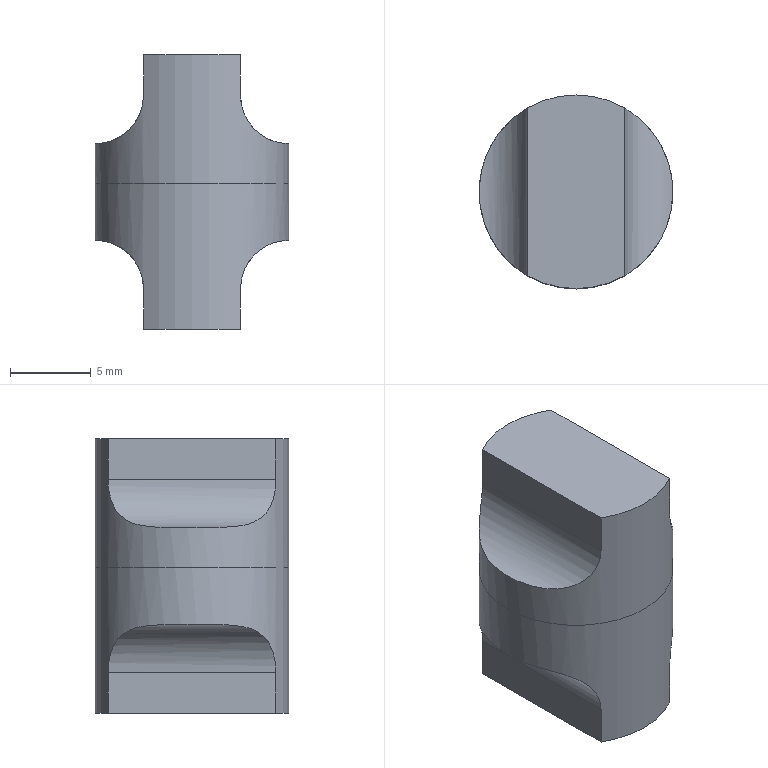NC program | NX | posted with a generic post | part box 12 x 12 x 17 mm
Lines 1210 to 2569 of 2569:
(PLANAR_MILL_COPY_1_COPY_COPY , TOOL : D8开粗)
N2328 T01 M6
N2330 G54
N2332 G17 G0 G90 X0. Y-12.196 S2000 M3
N2334 G43 Z20. H1
N2336 Z2.05
N2338 G94 G1 Z0.05 F800.
N2340 Y-5.196
N2342 Y5.196
N2344 Y12.196
N2346 Z2.05
N2348 G0 Z20.
(ADAPTIVE_MILLING_1_COPY , TOOL : D8开粗)
N2350 X-16.493 Y0.096 S2500
N2352 Z-6.994
N2354 G1 X-16.343 Z-7.931 F1000.
N2356 X-16.193 Z-8.301
N2358 X-16.043 Z-8.574
N2360 X-15.893 Z-8.794
N2362 X-15.743 Z-8.978
N2364 X-15.593 Z-9.136
N2366 X-15.443 Z-9.274
N2368 X-15.293 Z-9.394
N2370 X-15.143 Z-9.499
N2372 X-14.993 Z-9.592
N2374 X-14.843 Z-9.673
N2376 X-14.693 Z-9.743
N2378 X-14.543 Z-9.804
N2380 X-14.393 Z-9.856
N2382 X-14.243 Z-9.899
N2384 X-14.093 Z-9.933
N2386 X-13.943 Z-9.96
N2388 X-13.793 Z-9.979
N2390 X-13.643 Y0.095 Z-9.99
N2392 X-13.493 Z-9.994
N2394 X-12.229
N2396 G3 X-11.465 Y0.639 R0.809
N2398 G2 X-10.606 Y3.647 R33.117
N2400 X4.464 Y10.246 R11.261
N2402 X-11.107 Y-1.066 R-11.169
N2404 X-6.24 Y8.898 R11.713
N2406 X-10.604 Y-2.307 R-10.863
N2408 X-3.391 Y9.995 R11.018
N2410 X-10.105 Y-2.977 R-10.55
N2412 X-1.423 Y10.137 R10.58
N2414 X-9.548 Y-3.628 R-10.231
N2416 X-10.028 Y1.009 R9.78
N2418 X-9.875 Y2.002 R4.333
N2420 G1 X-9.695 Y2.83
N2422 G2 X-8.521 Y5.423 R11.812
N2424 X-6.668 Y7.586 R11.812
N2426 X-4.354 Y9.113 R11.863
N2428 X-0.441 Y10.09 R10.913
N2430 X3.543 Y9.458 R10.913
N2432 G1 X4.9 Y8.832
N2434 X6.149 Y8.012
N2436 X7.264 Y7.017
N2438 X8.22 Y5.868
N2440 X8.996 Y4.591
N2442 X9.575 Y3.213
N2444 X9.944 Y1.765
N2446 X10.096 Y0.279
N2448 X10.027 Y-1.214
N2450 X9.738 Y-2.68
N2452 X9.236 Y-4.088
N2454 X8.531 Y-5.406
N2456 X7.639 Y-6.607
N2458 X6.579 Y-7.663
N2460 G2 X5.058 Y-8.743 R18.614
N2462 G1 X3.65 Y-9.417
N2464 X2.174 Y-9.863
N2466 X0.646 Y-10.079
N2468 X-0.896 Y-10.06
N2470 X-2.418 Y-9.806
N2472 X-3.883 Y-9.323
N2474 X-5.258 Y-8.623
N2476 X-6.51 Y-7.722
N2478 X-7.61 Y-6.64
N2480 X-8.533 Y-5.404
N2482 G2 X-9.702 Y-2.808 R11.812
N2484 X-10.1 Y0.01 R11.818
N2486 G1 X-9.997 Y1.435
N2488 X-9.871 Y2.021
N2490 G3 X-10.332 Y2.931 R0.808
N2492 G1 X-11.574 Y3.482
N2494 X-11.711 Y3.543 Z-9.99
N2496 X-11.848 Y3.604 Z-9.979
N2498 X-11.985 Y3.665 Z-9.96
N2500 X-12.122 Y3.726 Z-9.933
N2502 X-12.259 Y3.787 Z-9.899
N2504 X-12.396 Y3.848 Z-9.856
N2506 X-12.534 Y3.909 Z-9.804
N2508 X-12.671 Y3.97 Z-9.743
N2510 X-12.808 Y4.031 Z-9.673
N2512 X-12.945 Y4.092 Z-9.592
N2514 X-13.082 Y4.152 Z-9.499
N2516 X-13.219 Y4.213 Z-9.394
N2518 X-13.356 Y4.274 Z-9.274
N2520 X-13.493 Y4.335 Z-9.136
N2522 X-13.63 Y4.396 Z-8.978
N2524 X-13.767 Y4.457 Z-8.794
N2526 X-13.904 Y4.518 Z-8.574
N2528 X-14.041 Y4.579 Z-8.301
N2530 X-14.178 Y4.64 Z-7.931
N2532 X-14.316 Y4.701 Z-6.994
N2534 G0 Z20.
N2536 X-10.972 Y-10.352
N2538 Z-1.997
N2540 G1 X-10.86 Y-10.252 Z-2.934
N2542 X-10.749 Y-10.151 Z-3.305
N2544 X-10.638 Y-10.051 Z-3.577
N2546 X-10.526 Y-9.95 Z-3.797
N2548 X-10.415 Y-9.85 Z-3.981
N2550 X-10.304 Y-9.749 Z-4.139
N2552 X-10.192 Y-9.649 Z-4.277
N2554 X-10.081 Y-9.548 Z-4.397
N2556 X-9.969 Y-9.448 Z-4.502
N2558 X-9.858 Y-9.347 Z-4.595
N2560 X-9.747 Y-9.247 Z-4.676
N2562 X-9.635 Y-9.146 Z-4.746
N2564 X-9.524 Y-9.046 Z-4.807
N2566 X-9.412 Y-8.945 Z-4.859
N2568 X-9.301 Y-8.845 Z-4.902
N2570 X-9.19 Y-8.745 Z-4.936
N2572 X-9.078 Y-8.644 Z-4.963
N2574 X-8.967 Y-8.544 Z-4.982
N2576 X-8.856 Y-8.443 Z-4.993
N2578 X-8.744 Y-8.343 Z-4.997
N2580 X-7.834 Y-7.521
N2582 G3 X-7.742 Y-6.419 R0.808
N2584 G2 X-9.589 Y-1.959 R13.939
N2586 X-8.36 Y5.047 R9.929
N2588 X-7.73 Y6.434 R4.2
N2590 G3 X-8.564 Y7.705 R0.8
N2592 X-8.986 Y7.449 Z-4.966 R1.078
N2594 G1 X-9.831 Y6.752 Z-4.897
N2596 X-10.469 Y6.225 F10000.
N2598 G3 X-10.759 Y5.623 R0.803
N2600 G1 X-10.954 Y-5.3
N2602 G3 X-10.641 Y-5.949 R0.802
N2604 G1 X-10.006 Y-6.437
N2606 X-9.072 Y-7.148 Z-4.971 F1000.
N2608 G3 X-8.68 Y-7.28 Z-4.997 R0.81
N2610 X-7.925 Y-6.112 R0.8
N2612 G2 X-8.398 Y-5.006 R5.111
N2614 X-9.449 Y-0.645 R13.912
N2616 X-8.524 Y4.104 R10.597
N2618 G1 X-8.442 Y4.768
N2620 X-8.35 Y5.08
N2622 G3 X-9.525 Y5.996 R0.8
N2624 X-9.874 Y5.607 Z-4.964 R1.031
N2626 G1 X-10.443 Y4.708 Z-4.897
N2628 X-10.724 Y4.27 F10000.
N2630 X-10.993 Y3.826
N2632 X-11.044 Y3.672
N2634 X-11.066 Y3.512
N2636 X-11.259 Y-4.672
N2638 G3 X-10.917 Y-5.348 R0.801
N2640 G1 X-10.213 Y-5.839
N2642 X-9.397 Y-6.401 Z-4.959 F1000.
N2644 G3 X-8.817 Y-6.491 Z-4.997 R0.801
N2646 X-8.23 Y-5.484 R0.8
N2648 G2 X-9.121 Y-1.322 R24.508
N2650 X-8.6 Y3.105 R11.126
N2652 G3 X-8.525 Y3.922 R2.117
N2654 G1 X-8.493 Y4.245
N2656 G3 X-9.346 Y5.121 R0.8
N2658 X-9.961 Y4.766 Z-4.951 R0.841
N2660 G1 X-10.501 Y4.098 Z-4.897
N2662 X-11.419 Y2.964 F10000.
N2664 G3 X-11.597 Y2.453 R0.807
N2666 G1 X-11.547 Y-2.973
N2668 G3 X-11.371 Y-3.467 R0.808
N2670 G1 X-10.47 Y-4.588
N2672 X-9.82 Y-5.389 Z-4.962 F1000.
N2674 G3 X-9.331 Y-5.638 Z-4.997 R0.802
N2676 X-8.443 Y-4.765 R0.8
N2678 X-8.829 Y-1.849 R153.035
N2680 G2 X-8.526 Y2.412 R13.535
N2682 G1 X-8.525 Y3.462
N2684 G3 X-9.318 Y4.262 R0.8
N2686 X-9.985 Y3.921 Z-4.948 R0.83
N2688 G1 X-10.51 Y3.297 Z-4.897
N2690 X-11.441 Y2.191 F10000.
N2692 G3 X-11.629 Y1.67 R0.807
N2694 G1 X-11.6 Y-2.426
N2696 G3 X-11.424 Y-2.922 R0.808
N2698 G1 X-10.519 Y-4.046
N2700 X-9.873 Y-4.843 Z-4.961 F1000.
N2702 G3 X-9.377 Y-5.091 Z-4.997 R0.802
N2704 X-8.496 Y-4.218 R0.8
N2706 G2 X-8.644 Y-0.765 R76.33
N2708 X-8.525 Y0.856 R32.63
N2710 G1 Y2.456
N2712 G3 X-9.901 Y3.011 R0.8
N2714 X-10.13 Y2.585 Z-4.966 R1.096
N2716 G1 X-10.512 Y1.549 Z-4.897
N2718 X-10.78 Y0.83 F10000.
N2720 X-11.037 Y0.108
N2722 X-11.059 Y-0.078
N2724 X-11.054 Y-1.156
N2726 X-11.01 Y-1.339
N2728 X-10.521 Y-2.665
N2730 X-10.284 Y-3.317 Z-4.941 F1000.
N2732 X-10.035 Y-3.966 Z-4.984
N2734 X-9.919 Y-4.132 Z-4.997
N2736 G3 X-8.525 Y-3.596 R0.8
N2738 G1 Y0.879
N2740 G3 X-9.442 Y1.679 R0.808
N2742 G1 X-10.516 Y1.533
N2744 X-10.665 Y1.513 Z-4.993
N2746 X-10.813 Y1.493 Z-4.982
N2748 X-10.962 Y1.473 Z-4.963
N2750 X-11.111 Y1.453 Z-4.936
N2752 X-11.259 Y1.432 Z-4.902
N2754 X-11.408 Y1.412 Z-4.859
N2756 X-11.557 Y1.392 Z-4.807
N2758 X-11.705 Y1.372 Z-4.746
N2760 X-11.854 Y1.352 Z-4.676
N2762 X-12.002 Y1.331 Z-4.595
N2764 X-12.151 Y1.311 Z-4.502
N2766 X-12.3 Y1.291 Z-4.397
N2768 X-12.448 Y1.271 Z-4.277
N2770 X-12.597 Y1.251 Z-4.139
N2772 X-12.746 Y1.23 Z-3.981
N2774 X-12.894 Y1.21 Z-3.797
N2776 X-13.043 Y1.19 Z-3.577
N2778 X-13.192 Y1.17 Z-3.305
N2780 X-13.34 Y1.15 Z-2.934
N2782 X-13.489 Y1.129 Z-1.997
N2784 G0 Z20.
N2786 X-9.475 Y-11.737
N2788 Z-1.497
N2790 G1 X-9.375 Y-11.625 Z-2.434
N2792 X-9.276 Y-11.513 Z-2.805
N2794 X-9.176 Y-11.4 Z-3.078
N2796 X-9.077 Y-11.288 Z-3.297
N2798 X-8.977 Y-11.176 Z-3.482
N2800 X-8.878 Y-11.064 Z-3.64
N2802 X-8.778 Y-10.951 Z-3.777
N2804 X-8.679 Y-10.839 Z-3.897
N2806 X-8.579 Y-10.727 Z-4.003
N2808 X-8.48 Y-10.615 Z-4.095
N2810 X-8.38 Y-10.502 Z-4.176
N2812 X-8.281 Y-10.39 Z-4.247
N2814 X-8.181 Y-10.278 Z-4.307
N2816 X-8.082 Y-10.166 Z-4.359
N2818 X-7.982 Y-10.053 Z-4.402
N2820 X-7.883 Y-9.941 Z-4.437
N2822 X-7.783 Y-9.829 Z-4.463
N2824 X-7.684 Y-9.717 Z-4.482
N2826 X-7.584 Y-9.604 Z-4.493
N2828 X-7.485 Y-9.492 Z-4.497
N2830 X-6.685 Y-8.59
N2832 G3 X-6.715 Y-7.485 R0.808
N2834 G2 X-7.319 Y-6.688 R2.318
N2836 X-7.956 Y-5.009 R4.7
N2838 X-8.305 Y-0.981 R20.194
N2840 X-8.294 Y3.368 R73.56
N2842 X-7.844 Y5.104 R8.09
N2844 G3 X-8.82 Y5.995 R0.8
N2846 X-9.34 Y5.606 Z-4.455 R0.845
N2848 G1 X-9.864 Y4.843 Z-4.397
N2850 X-10.421 Y4.031 F10000.
N2852 G3 X-10.56 Y3.536 R0.808
N2854 G1 X-10.04 Y-6.375
N2856 G3 X-9.749 Y-6.952 R0.803
N2858 G1 X-9.241 Y-7.369
N2860 X-8.149 Y-8.26 Z-4.486 F1000.
N2862 X-7.99 Y-8.35 Z-4.497
N2864 G3 X-7.011 Y-7.187 R0.8
N2866 G1 X-7.505 Y-6.386
N2868 X-7.806 Y-5.494
N2870 G2 X-8.077 Y2.553 R57.283
N2872 G1 X-7.897 Y3.789
N2874 G2 X-7.805 Y5.494 R10.044
N2876 G1 X-7.504 Y6.386
N2878 X-7.01 Y7.187
N2880 X-6.711 Y7.489
N2882 G3 X-7.805 Y8.655 R0.8
N2884 G1 X-7.97 Y8.512
N2886 X-9.172 Y7.467 Z-4.397
N2888 X-9.367 Y7.299 F10000.
N2890 X-9.554 Y7.122
N2892 G3 X-9.74 Y6.677 R0.811
N2894 G1 X-10.613 Y-2.984
N2896 G3 X-10.457 Y-3.535 R0.806
N2898 G1 X-9.902 Y-4.277
N2900 X-9.295 Y-5.08 Z-4.46 F1000.
N2902 G3 X-8.788 Y-5.347 Z-4.497 R0.801
N2904 X-7.897 Y-4.552 R0.8
N2906 G1 Y3.798
N2908 G3 X-8.545 Y4.59 R0.808
N2910 G1 X-9.869 Y4.858
N2912 X-10.016 Y4.887 Z-4.493
N2914 X-10.163 Y4.917 Z-4.482
N2916 X-10.31 Y4.947 Z-4.463
N2918 X-10.457 Y4.976 Z-4.437
N2920 X-10.604 Y5.006 Z-4.402
N2922 X-10.751 Y5.036 Z-4.359
N2924 X-10.898 Y5.065 Z-4.307
N2926 X-11.045 Y5.095 Z-4.247
N2928 X-11.192 Y5.125 Z-4.176
N2930 X-11.339 Y5.155 Z-4.095
N2932 X-11.486 Y5.184 Z-4.003
N2934 X-11.633 Y5.214 Z-3.897
N2936 X-11.78 Y5.244 Z-3.777
N2938 X-11.927 Y5.273 Z-3.64
N2940 X-12.074 Y5.303 Z-3.482
N2942 X-12.221 Y5.333 Z-3.297
N2944 X-12.368 Y5.362 Z-3.078
N2946 X-12.515 Y5.392 Z-2.805
N2948 X-12.662 Y5.422 Z-2.434
N2950 X-12.809 Y5.452 Z-1.497
N2952 G0 Z20.
N2954 X-9.023 Y-12.067
N2956 Z-0.998
N2958 G1 X-8.923 Y-11.955 Z-1.934
N2960 X-8.823 Y-11.843 Z-2.305
N2962 X-8.724 Y-11.731 Z-2.578
N2964 X-8.624 Y-11.619 Z-2.798
N2966 X-8.524 Y-11.508 Z-2.982
N2968 X-8.424 Y-11.396 Z-3.14
N2970 X-8.324 Y-11.284 Z-3.277
N2972 X-8.224 Y-11.172 Z-3.398
N2974 X-8.124 Y-11.06 Z-3.503
N2976 X-8.024 Y-10.948 Z-3.596
N2978 X-7.924 Y-10.836 Z-3.677
N2980 X-7.824 Y-10.724 Z-3.747
N2982 X-7.724 Y-10.613 Z-3.808
N2984 X-7.624 Y-10.501 Z-3.859
N2986 X-7.525 Y-10.389 Z-3.902
N2988 X-7.425 Y-10.277 Z-3.937
N2990 X-7.325 Y-10.165 Z-3.964
N2992 X-7.225 Y-10.053 Z-3.982
N2994 X-7.125 Y-9.941 Z-3.994
N2996 X-7.025 Y-9.829 Z-3.998
N2998 X-6.254 Y-8.966
N3000 G3 X-6.339 Y-7.808 R0.808
N3002 G2 X-7.552 Y-4.89 R4.516
N3004 X-7.693 Y1.156 R74.364
N3006 X-7.658 Y4.005 R35.287
N3008 G3 X-7.447 Y5.686 R10.663
N3010 G2 X-6.324 Y7.82 R4.364
N3012 G3 X-7.358 Y9.043 R-0.801
N3014 G1 X-8.62 Y8.071 Z-3.898
N3016 X-9.483 Y7.408 F10000.
N3018 G3 X-9.786 Y6.892 R0.805
N3020 X-10.088 Y4.601 R34.73
N3022 G1 X-10.134 Y3.943
N3024 X-10.552 Y-3.891
N3026 G3 X-10.369 Y-4.444 R0.805
N3028 G1 X-9.473 Y-5.524
N3030 X-8.817 Y-6.307 Z-3.962 F1000.
N3032 G3 X-8.313 Y-6.548 Z-3.998 R0.802
N3034 X-7.448 Y-5.683 R0.8
N3036 G1 X-7.517 Y-4.876
N3038 Y4.799
N3040 G3 X-8.331 Y5.607 R0.808
N3042 G1 X-9.453 Y5.599
N3044 X-9.603 Y5.597 Z-3.994
N3046 X-9.753 Y5.596 Z-3.982
N3048 X-9.903 Y5.595 Z-3.964
N3050 X-10.053 Y5.594 Z-3.937
N3052 X-10.203 Y5.593 Z-3.902
N3054 X-10.353 Y5.592 Z-3.859
N3056 X-10.503 Y5.59 Z-3.808
N3058 X-10.653 Y5.589 Z-3.747
N3060 X-10.803 Y5.588 Z-3.677
N3062 X-10.953 Y5.587 Z-3.596
N3064 X-11.103 Y5.586 Z-3.503
N3066 X-11.253 Y5.585 Z-3.398
N3068 X-11.403 Y5.584 Z-3.277
N3070 X-11.553 Y5.582 Z-3.14
N3072 X-11.703 Y5.581 Z-2.982
N3074 X-11.853 Y5.58 Z-2.798
N3076 X-12.003 Y5.579 Z-2.578
N3078 X-12.153 Y5.578 Z-2.305
N3080 X-12.303 Y5.577 Z-1.934
N3082 X-12.453 Y5.575 Z-0.998
N3084 G0 Z20.
N3086 X-8.334 Y-12.558
N3088 Z-0.498
N3090 G1 X-8.252 Y-12.433 Z-1.435
N3092 X-8.169 Y-12.307 Z-1.806
N3094 X-8.087 Y-12.182 Z-2.078
N3096 X-8.004 Y-12.057 Z-2.298
N3098 X-7.922 Y-11.931 Z-2.482
N3100 X-7.84 Y-11.806 Z-2.64
N3102 X-7.757 Y-11.681 Z-2.778
N3104 X-7.675 Y-11.555 Z-2.898
N3106 X-7.592 Y-11.43 Z-3.003
N3108 X-7.51 Y-11.304 Z-3.096
N3110 X-7.428 Y-11.179 Z-3.177
N3112 X-7.345 Y-11.054 Z-3.247
N3114 X-7.263 Y-10.928 Z-3.308
N3116 X-7.18 Y-10.803 Z-3.36
N3118 X-7.098 Y-10.678 Z-3.403
N3120 X-7.016 Y-10.552 Z-3.437
N3122 X-6.933 Y-10.427 Z-3.464
N3124 X-6.851 Y-10.302 Z-3.483
N3126 X-6.768 Y-10.176 Z-3.494
N3128 X-6.686 Y-10.051 Z-3.498
N3130 X-5.986 Y-8.986
N3132 G3 X-6.05 Y-8.014 R0.808
N3134 G2 X-7.198 Y-5.919 R4.296
N3136 X-7.309 Y-3.005 R24.055
N3138 X-7.296 Y4.125 R272.34
N3140 G3 X-7.283 Y5.091 R35.242
N3142 G2 X-6.548 Y7.436 R4.382
N3144 G1 X-6.041 Y8.022
N3146 G3 X-7.164 Y9.156 R0.8
N3148 G1 X-8.413 Y8.169 Z-3.398
N3150 X-9.223 Y7.528 F10000.
N3152 G3 X-9.503 Y7.095 R0.808
N3154 G1 X-9.624 Y6.613
N3156 X-9.715 Y6.125
N3158 X-9.736 Y5.879
N3160 X-9.748 Y5.631
N3162 X-9.811 Y-2.556
N3164 X-9.798 Y-2.7
N3166 X-9.762 Y-2.84
N3168 X-9.275 Y-4.157
N3170 X-9.036 Y-4.81 Z-3.442 F1000.
N3172 X-8.787 Y-5.46 Z-3.485
N3174 X-8.672 Y-5.625 Z-3.498
N3176 G3 X-7.277 Y-5.09 R0.8
N3178 G1 Y4.335
N3180 G3 X-7.914 Y5.124 R0.808
N3182 G1 X-9.252 Y5.413
N3184 X-9.398 Y5.445 Z-3.494
N3186 X-9.545 Y5.477 Z-3.483
N3188 X-9.692 Y5.509 Z-3.464
N3190 X-9.838 Y5.54 Z-3.437
N3192 X-9.985 Y5.572 Z-3.403
N3194 X-10.131 Y5.604 Z-3.36
N3196 X-10.278 Y5.635 Z-3.308
N3198 X-10.425 Y5.667 Z-3.247
N3200 X-10.571 Y5.699 Z-3.177
N3202 X-10.718 Y5.73 Z-3.096
N3204 X-10.865 Y5.762 Z-3.003
N3206 X-11.011 Y5.794 Z-2.898
N3208 X-11.158 Y5.826 Z-2.778
N3210 X-11.304 Y5.857 Z-2.64
N3212 X-11.451 Y5.889 Z-2.482
N3214 X-11.598 Y5.921 Z-2.298
N3216 X-11.744 Y5.952 Z-2.078
N3218 X-11.891 Y5.984 Z-1.806
N3220 X-12.037 Y6.016 Z-1.435
N3222 X-12.184 Y6.047 Z-0.498
N3224 G0 Z20.
N3226 X-8.576 Y-12.367
N3228 Z0.002
N3230 G1 X-8.488 Y-12.246 Z-0.935
N3232 X-8.399 Y-12.125 Z-1.306
N3234 X-8.311 Y-12.004 Z-1.578
N3236 X-8.222 Y-11.883 Z-1.798
N3238 X-8.134 Y-11.762 Z-1.982
N3240 X-8.045 Y-11.641 Z-2.141
N3242 X-7.957 Y-11.52 Z-2.278
N3244 X-7.868 Y-11.399 Z-2.398
N3246 X-7.78 Y-11.277 Z-2.504
N3248 X-7.691 Y-11.156 Z-2.596
N3250 X-7.603 Y-11.035 Z-2.677
N3252 X-7.514 Y-10.914 Z-2.748
N3254 X-7.426 Y-10.793 Z-2.808
N3256 X-7.337 Y-10.672 Z-2.86
N3258 X-7.248 Y-10.551 Z-2.903
N3260 X-7.16 Y-10.43 Z-2.938
N3262 X-7.071 Y-10.309 Z-2.964
N3264 X-6.983 Y-10.188 Z-2.983
N3266 X-6.894 Y-10.067 Z-2.994
N3268 X-6.806 Y-9.945 Z-2.998
N3270 X-6.051 Y-8.913
N3272 G3 X-6.095 Y-7.904 R0.808
N3274 G2 X-6.828 Y-6.801 R4.039
N3276 X-7.143 Y-5.17 R4.585
N3278 G1 Y5.167
N3280 G2 X-6.39 Y7.57 R4.301
N3282 G1 X-6.039 Y7.96
N3284 G3 X-5.984 Y8.972 R0.808
N3286 G1 X-6.726 Y10.005
N3288 X-6.813 Y10.127 Z-2.994
N3290 X-6.901 Y10.248 Z-2.983
N3292 X-6.988 Y10.37 Z-2.964
N3294 X-7.076 Y10.492 Z-2.938
N3296 X-7.163 Y10.614 Z-2.903
N3298 X-7.251 Y10.736 Z-2.86
N3300 X-7.339 Y10.857 Z-2.808
N3302 X-7.426 Y10.979 Z-2.748
N3304 X-7.514 Y11.101 Z-2.677
N3306 X-7.601 Y11.223 Z-2.596
N3308 X-7.689 Y11.345 Z-2.504
N3310 X-7.776 Y11.466 Z-2.398
N3312 X-7.864 Y11.588 Z-2.278
N3314 X-7.951 Y11.71 Z-2.141
N3316 X-8.039 Y11.832 Z-1.982
N3318 X-8.126 Y11.954 Z-1.798
N3320 X-8.214 Y12.075 Z-1.578
N3322 X-8.302 Y12.197 Z-1.306
N3324 X-8.389 Y12.319 Z-0.935
N3326 X-8.477 Y12.441 Z0.002
N3328 G0 Z20.
N3330 X-9.088 Y-11.906
N3332 Z0.502
N3334 G1 X-8.999 Y-11.785 Z-0.435
N3336 X-8.91 Y-11.664 Z-0.806
N3338 X-8.822 Y-11.543 Z-1.079
N3340 X-8.733 Y-11.422 Z-1.298
N3342 X-8.644 Y-11.301 Z-1.483
N3344 X-8.555 Y-11.18 Z-1.641
N3346 X-8.467 Y-11.059 Z-1.778
N3348 X-8.378 Y-10.938 Z-1.898
N3350 X-8.289 Y-10.817 Z-2.004
N3352 X-8.2 Y-10.696 Z-2.097
N3354 X-8.112 Y-10.575 Z-2.178
N3356 X-8.023 Y-10.454 Z-2.248
N3358 X-7.934 Y-10.333 Z-2.309
N3360 X-7.846 Y-10.212 Z-2.36
N3362 X-7.757 Y-10.092 Z-2.403
N3364 X-7.668 Y-9.971 Z-2.438
N3366 X-7.579 Y-9.85 Z-2.465
N3368 X-7.491 Y-9.729 Z-2.483
N3370 X-7.402 Y-9.608 Z-2.495
N3372 X-7.313 Y-9.487 Z-2.498
N3374 X-6.462 Y-8.327
N3376 G3 X-6.411 Y-7.45 R0.809
N3378 G2 X-7.1 Y-5.218 R4.194
N3380 G1 Y5.223
N3382 G2 X-6.404 Y7.465 R4.309
N3384 G3 X-6.454 Y8.335 R0.809
N3386 G1 X-7.3 Y9.502
N3388 X-7.387 Y9.623 Z-2.495
N3390 X-7.475 Y9.745 Z-2.483
N3392 X-7.563 Y9.866 Z-2.465
N3394 X-7.651 Y9.988 Z-2.438
N3396 X-7.739 Y10.109 Z-2.403
N3398 X-7.827 Y10.231 Z-2.36
N3400 X-7.915 Y10.352 Z-2.309
N3402 X-8.003 Y10.474 Z-2.248
N3404 X-8.091 Y10.595 Z-2.178
N3406 X-8.179 Y10.717 Z-2.097
N3408 X-8.267 Y10.838 Z-2.004
N3410 X-8.355 Y10.96 Z-1.898
N3412 X-8.443 Y11.081 Z-1.778
N3414 X-8.531 Y11.203 Z-1.641
N3416 X-8.619 Y11.324 Z-1.483
N3418 X-8.707 Y11.445 Z-1.298
N3420 X-8.795 Y11.567 Z-1.079
N3422 X-8.883 Y11.688 Z-0.806
N3424 X-8.971 Y11.81 Z-0.435
N3426 X-9.059 Y11.931 Z0.502
N3428 G0 Z20.
N3430 X11.085 Y10.228
N3432 Z-1.997
N3434 G1 X10.972 Y10.13 Z-2.934
N3436 X10.858 Y10.032 Z-3.305
N3438 X10.745 Y9.934 Z-3.577
N3440 X10.631 Y9.836 Z-3.797
N3442 X10.518 Y9.738 Z-3.981
N3444 X10.404 Y9.64 Z-4.139
N3446 X10.291 Y9.542 Z-4.277
N3448 X10.177 Y9.444 Z-4.397
N3450 X10.064 Y9.345 Z-4.502
N3452 X9.95 Y9.247 Z-4.595
N3454 X9.837 Y9.149 Z-4.676
N3456 X9.723 Y9.051 Z-4.746
N3458 X9.61 Y8.953 Z-4.807
N3460 X9.496 Y8.855 Z-4.859
N3462 X9.383 Y8.757 Z-4.902
N3464 X9.269 Y8.659 Z-4.936
N3466 X9.156 Y8.561 Z-4.963
N3468 X9.042 Y8.463 Z-4.982
N3470 X8.929 Y8.365 Z-4.993
N3472 X8.815 Y8.266 Z-4.997
N3474 X7.9 Y7.475
N3476 G3 X7.799 Y6.357 R0.808
N3478 G2 X9.371 Y2.861 R17.116
N3480 X8.371 Y-5.033 R9.98
N3482 X7.788 Y-6.371 R4.49
N3484 G3 X8.591 Y-7.653 R0.8
N3486 X9.038 Y-7.392 Z-4.964 R1.037
N3488 G1 X9.861 Y-6.71 Z-4.897
N3490 X10.528 Y-6.158 F10000.
N3492 G3 X10.817 Y-5.56 R0.803
N3494 G1 X11.056 Y5.117
N3496 G3 X10.744 Y5.77 R0.802
N3498 G1 X10.079 Y6.28
N3500 X9.168 Y6.973 Z-4.969 F1000.
N3502 G3 X8.746 Y7.103 Z-4.997 R0.806
N3504 X8.027 Y5.929 R0.8
N3506 G2 X8.382 Y5.054 R4.155
N3508 X9.446 Y0.671 R14.288
N3510 X8.527 Y-4.102 R10.662
N3512 G1 X8.438 Y-4.815
N3514 X8.365 Y-5.054
N3516 G3 X9.523 Y-5.985 R0.8
N3518 X9.886 Y-5.589 Z-4.963 R1.01
N3520 G1 X10.446 Y-4.703 Z-4.897
N3522 X10.733 Y-4.254 F10000.
N3524 X11.009 Y-3.799
N3526 X11.059 Y-3.646
N3528 X11.081 Y-3.486
N3530 X11.283 Y4.608
N3532 G3 X10.942 Y5.283 R0.801
N3534 G1 X10.238 Y5.776
N3536 X9.42 Y6.341 Z-4.959 F1000.
N3538 G3 X8.843 Y6.433 Z-4.997 R0.801
N3540 X8.254 Y5.42 R0.8
N3542 G2 X9.12 Y1.322 R24.878
N3544 X8.6 Y-3.108 R11.179
N3546 G3 X8.525 Y-3.984 R2.25
N3548 G1 X8.499 Y-4.233
N3550 G3 X9.348 Y-5.115 R0.8
N3552 X9.966 Y-4.759 Z-4.951 R0.841
N3554 G1 X10.504 Y-4.093 Z-4.897
N3556 X11.425 Y-2.953 F10000.
N3558 G3 X11.603 Y-2.441 R0.807
N3560 G1 X11.542 Y3.02
N3562 G3 X11.367 Y3.511 R0.808
N3564 G1 X10.468 Y4.634
N3566 X9.816 Y5.44 Z-4.962 F1000.
N3568 G3 X9.333 Y5.689 Z-4.997 R0.802
N3570 X8.438 Y4.812 R0.8
N3572 X8.825 Y1.875 R184.936
N3574 G2 X8.526 Y-2.424 R13.724
N3576 G1 X8.525 Y-3.466
N3578 G3 X9.319 Y-4.266 R0.8
N3580 X9.985 Y-3.924 Z-4.948 R0.83
N3582 G1 X10.51 Y-3.3 Z-4.897
N3584 X11.441 Y-2.192 F10000.
N3586 G3 X11.629 Y-1.674 R0.807
N3588 G1 X11.612 Y2.349
N3590 G3 X11.436 Y2.846 R0.807
N3592 G1 X10.525 Y3.981
N3594 X9.884 Y4.771 Z-4.961 F1000.
N3596 G3 X9.381 Y5.02 Z-4.997 R0.801
N3598 X8.509 Y4.141 R0.8
N3600 G2 X8.646 Y0.926 R166.962
N3602 X8.525 Y-0.863 R24.532
N3604 G1 Y-2.463
N3606 G3 X9.901 Y-3.018 R0.8
N3608 X10.13 Y-2.592 Z-4.966 R1.096
N3610 G1 X10.512 Y-1.555 Z-4.897
N3612 X10.78 Y-0.837 F10000.
N3614 X11.037 Y-0.115
N3616 X11.059 Y0.071
N3618 X11.054 Y1.167
N3620 X11.01 Y1.35
N3622 X10.521 Y2.676
N3624 X10.284 Y3.329 Z-4.941 F1000.
N3626 X10.035 Y3.977 Z-4.984
N3628 X9.919 Y4.144 Z-4.997
N3630 G3 X8.525 Y3.608 R0.8
N3632 G1 Y-0.867
N3634 G3 X9.445 Y-1.668 R0.808
N3636 G1 X10.516 Y-1.518
N3638 X10.665 Y-1.497 Z-4.993
N3640 X10.813 Y-1.476 Z-4.982
N3642 X10.962 Y-1.456 Z-4.963
N3644 X11.11 Y-1.435 Z-4.936
N3646 X11.259 Y-1.414 Z-4.902
N3648 X11.407 Y-1.393 Z-4.859
N3650 X11.556 Y-1.373 Z-4.807
N3652 X11.705 Y-1.352 Z-4.746
N3654 X11.853 Y-1.331 Z-4.676
N3656 X12.002 Y-1.31 Z-4.595
N3658 X12.15 Y-1.289 Z-4.502
N3660 X12.299 Y-1.269 Z-4.397
N3662 X12.447 Y-1.248 Z-4.277
N3664 X12.596 Y-1.227 Z-4.139
N3666 X12.744 Y-1.206 Z-3.981
N3668 X12.893 Y-1.186 Z-3.797
N3670 X13.042 Y-1.165 Z-3.577
N3672 X13.19 Y-1.144 Z-3.305
N3674 X13.339 Y-1.123 Z-2.934
N3676 X13.487 Y-1.103 Z-1.997
N3678 G0 Z20.
N3680 X9.447 Y11.759
N3682 Z-1.497
N3684 G1 X9.348 Y11.647 Z-2.434
N3686 X9.249 Y11.534 Z-2.805
N3688 X9.15 Y11.421 Z-3.078
N3690 X9.051 Y11.308 Z-3.297
N3692 X8.952 Y11.196 Z-3.482
N3694 X8.853 Y11.083 Z-3.64
N3696 X8.754 Y10.97 Z-3.777
N3698 X8.656 Y10.857 Z-3.897
N3700 X8.557 Y10.744 Z-4.003
N3702 X8.458 Y10.632 Z-4.095
N3704 X8.359 Y10.519 Z-4.176
N3706 X8.26 Y10.406 Z-4.247
N3708 X8.161 Y10.293 Z-4.307
N3710 X8.062 Y10.181 Z-4.359
N3712 X7.963 Y10.068 Z-4.402
N3714 X7.864 Y9.955 Z-4.437
N3716 X7.765 Y9.842 Z-4.463
N3718 X7.667 Y9.729 Z-4.482
N3720 X7.568 Y9.617 Z-4.493
N3722 X7.469 Y9.504 Z-4.497
N3724 X6.672 Y8.595
N3726 G3 X6.704 Y7.495 R0.808
N3728 G2 X7.323 Y6.676 R2.383
N3730 X7.954 Y5.01 R4.722
N3732 X8.304 Y1.057 R19.829
N3734 X8.298 Y-3.342 R85.798
N3736 X7.845 Y-5.103 R7.847
N3738 G3 X8.82 Y-6.001 R0.8
N3740 X9.34 Y-5.61 Z-4.455 R0.845
N3742 G1 X9.862 Y-4.847 Z-4.397
N3744 X10.422 Y-4.029 F10000.
N3746 G3 X10.561 Y-3.535 R0.808
N3748 G1 X10.038 Y6.374
N3750 G3 X9.747 Y6.95 R0.803
N3752 G1 X9.238 Y7.369
N3754 X8.147 Y8.259 Z-4.486 F1000.
N3756 X7.987 Y8.349 Z-4.497
N3758 G3 X7.009 Y7.186 R0.8
N3760 G1 X7.503 Y6.385
N3762 X7.804 Y5.493
N3764 G2 X8.079 Y-2.53 R58.435
N3766 G1 X7.897 Y-3.791
N3768 G2 X7.806 Y-5.495 R10.321
N3770 G1 X7.505 Y-6.387
N3772 X7.011 Y-7.188
N3774 X6.711 Y-7.489
N3776 G3 X7.804 Y-8.656 R0.8
N3778 G1 X7.972 Y-8.51
N3780 X9.174 Y-7.465 Z-4.397
N3782 X9.368 Y-7.298 F10000.
N3784 X9.555 Y-7.122
N3786 G3 X9.741 Y-6.677 R0.811
N3788 G1 X10.613 Y2.984
N3790 G3 X10.457 Y3.535 R0.806
N3792 G1 X9.902 Y4.277
N3794 X9.295 Y5.08 Z-4.46 F1000.
N3796 G3 X8.788 Y5.347 Z-4.497 R0.801
N3798 X7.897 Y4.552 R0.8
N3800 G1 Y-3.798
N3802 G3 X8.545 Y-4.59 R0.808
N3804 G1 X9.868 Y-4.857
N3806 X10.015 Y-4.887 Z-4.493
N3808 X10.162 Y-4.917 Z-4.482
N3810 X10.309 Y-4.947 Z-4.463
N3812 X10.456 Y-4.976 Z-4.437
N3814 X10.603 Y-5.006 Z-4.402
N3816 X10.75 Y-5.036 Z-4.359
N3818 X10.897 Y-5.065 Z-4.307
N3820 X11.044 Y-5.095 Z-4.247
N3822 X11.191 Y-5.125 Z-4.176
N3824 X11.338 Y-5.154 Z-4.095
N3826 X11.485 Y-5.184 Z-4.003
N3828 X11.632 Y-5.214 Z-3.897
N3830 X11.779 Y-5.244 Z-3.777
N3832 X11.926 Y-5.273 Z-3.64
N3834 X12.073 Y-5.303 Z-3.482
N3836 X12.22 Y-5.333 Z-3.297
N3838 X12.367 Y-5.362 Z-3.078
N3840 X12.514 Y-5.392 Z-2.805
N3842 X12.661 Y-5.422 Z-2.434
N3844 X12.808 Y-5.451 Z-1.497
N3846 G0 Z20.
N3848 X9.021 Y12.069
N3850 Z-0.998
N3852 G1 X8.921 Y11.957 Z-1.934
N3854 X8.821 Y11.845 Z-2.305
N3856 X8.722 Y11.733 Z-2.578
N3858 X8.622 Y11.621 Z-2.798
N3860 X8.522 Y11.509 Z-2.982
N3862 X8.423 Y11.397 Z-3.14
N3864 X8.323 Y11.284 Z-3.277
N3866 X8.223 Y11.172 Z-3.398
N3868 X8.124 Y11.06 Z-3.503
N3870 X8.024 Y10.948 Z-3.596
N3872 X7.924 Y10.836 Z-3.677
N3874 X7.825 Y10.724 Z-3.747
N3876 X7.725 Y10.612 Z-3.808
N3878 X7.625 Y10.5 Z-3.859
N3880 X7.526 Y10.388 Z-3.902
N3882 X7.426 Y10.276 Z-3.937
N3884 X7.326 Y10.164 Z-3.964
N3886 X7.227 Y10.051 Z-3.982
N3888 X7.127 Y9.939 Z-3.994
N3890 X7.027 Y9.827 Z-3.998
N3892 X6.258 Y8.962
N3894 G3 X6.344 Y7.804 R0.808
N3896 G2 X7.552 Y4.89 R4.507
N3898 X7.687 Y-0.106 R61.649
N3900 X7.666 Y-3.905 R80.374
N3902 G3 X7.449 Y-5.687 R13.252
N3904 G2 X6.345 Y-7.805 R4.383
N3906 G3 X7.53 Y-8.879 R0.801
N3908 G1 X8.743 Y-7.846 Z-3.898
N3910 X8.969 Y-7.657 F10000.
N3912 X9.185 Y-7.456
N3914 G3 X9.374 Y-6.993 R0.81
N3916 G1 X10.165 Y4.115
N3918 G3 X10.019 Y4.636 R0.807
N3920 G1 X9.481 Y5.394
N3922 X8.861 Y6.259 Z-3.964 F1000.
N3924 G3 X8.42 Y6.531 Z-3.998 R0.804
N3926 X7.449 Y5.683 R0.8
N3928 G1 X7.517 Y4.876
N3930 Y-4.799
N3932 G3 X8.33 Y-5.607 R0.808
N3934 G1 X9.454 Y-5.6
N3936 X9.604 Y-5.598 Z-3.994
N3938 X9.754 Y-5.597 Z-3.982
N3940 X9.904 Y-5.596 Z-3.964
N3942 X10.054 Y-5.595 Z-3.937
N3944 X10.204 Y-5.594 Z-3.902
N3946 X10.354 Y-5.593 Z-3.859
N3948 X10.504 Y-5.592 Z-3.808
N3950 X10.654 Y-5.591 Z-3.747
N3952 X10.804 Y-5.59 Z-3.677
N3954 X10.954 Y-5.589 Z-3.596
N3956 X11.104 Y-5.588 Z-3.503
N3958 X11.254 Y-5.587 Z-3.398
N3960 X11.404 Y-5.586 Z-3.277
N3962 X11.554 Y-5.585 Z-3.14
N3964 X11.704 Y-5.584 Z-2.982
N3966 X11.854 Y-5.583 Z-2.798
N3968 X12.004 Y-5.582 Z-2.578
N3970 X12.154 Y-5.581 Z-2.305
N3972 X12.304 Y-5.58 Z-1.934
N3974 X12.454 Y-5.579 Z-0.998
N3976 G0 Z20.
N3978 X8.471 Y12.467
N3980 Z-0.498
N3982 G1 X8.386 Y12.343 Z-1.435
N3984 X8.302 Y12.219 Z-1.806
N3986 X8.217 Y12.095 Z-2.078
N3988 X8.133 Y11.971 Z-2.298
N3990 X8.048 Y11.847 Z-2.482
N3992 X7.964 Y11.723 Z-2.64
N3994 X7.879 Y11.599 Z-2.778
N3996 X7.795 Y11.475 Z-2.898
N3998 X7.71 Y11.351 Z-3.003
N4000 X7.626 Y11.228 Z-3.096
N4002 X7.541 Y11.104 Z-3.177
N4004 X7.457 Y10.98 Z-3.247
N4006 X7.372 Y10.856 Z-3.308
N4008 X7.288 Y10.732 Z-3.36
N4010 X7.203 Y10.608 Z-3.403
N4012 X7.119 Y10.484 Z-3.437
N4014 X7.034 Y10.36 Z-3.464
N4016 X6.95 Y10.236 Z-3.483
N4018 X6.865 Y10.112 Z-3.494
N4020 X6.781 Y9.988 Z-3.498
N4022 X6.063 Y8.935
N4024 G3 X6.113 Y7.959 R0.808
N4026 G2 X7.277 Y5.155 R4.114
N4028 X7.301 Y-4.082 R433.946
N4030 G3 X7.277 Y-5.134 R17.687
N4032 G2 X6.065 Y-8.006 R4.171
N4034 G3 X7.172 Y-9.151 R0.8
N4036 G1 X8.422 Y-8.164 Z-3.398
N4038 X9.247 Y-7.512 F10000.
N4040 G3 X9.527 Y-7.078 R0.808
N4042 G1 X9.648 Y-6.597
N4044 X9.739 Y-6.109
N4046 X9.76 Y-5.862
N4048 X9.771 Y-5.615
N4050 X9.811 Y2.62
N4052 X9.797 Y2.763
N4054 X9.762 Y2.901
N4056 X9.274 Y4.222
N4058 X9.036 Y4.875 Z-3.442 F1000.
N4060 X8.787 Y5.524 Z-3.485
N4062 X8.672 Y5.69 Z-3.498
N4064 G3 X7.277 Y5.155 R0.8
N4066 G1 Y-4.345
N4068 G3 X7.915 Y-5.135 R0.808
N4070 G1 X9.249 Y-5.422
N4072 X9.396 Y-5.454 Z-3.494
N4074 X9.542 Y-5.486 Z-3.483
N4076 X9.689 Y-5.517 Z-3.464
N4078 X9.836 Y-5.549 Z-3.437
N4080 X9.982 Y-5.58 Z-3.403
N4082 X10.129 Y-5.612 Z-3.36
N4084 X10.276 Y-5.644 Z-3.308
N4086 X10.422 Y-5.675 Z-3.247
N4088 X10.569 Y-5.707 Z-3.177
N4090 X10.716 Y-5.738 Z-3.096
N4092 X10.862 Y-5.77 Z-3.003
N4094 X11.009 Y-5.801 Z-2.898
N4096 X11.155 Y-5.833 Z-2.778
N4098 X11.302 Y-5.865 Z-2.64
N4100 X11.449 Y-5.896 Z-2.482
N4102 X11.595 Y-5.928 Z-2.298
N4104 X11.742 Y-5.959 Z-2.078
N4106 X11.889 Y-5.991 Z-1.806
N4108 X12.035 Y-6.023 Z-1.435
N4110 X12.182 Y-6.054 Z-0.498
N4112 G0 Z20.
N4114 X8.352 Y12.532
N4116 Z0.002
N4118 G1 X8.265 Y12.409 Z-0.935
N4120 X8.179 Y12.287 Z-1.306
N4122 X8.092 Y12.164 Z-1.578
N4124 X8.006 Y12.042 Z-1.798
N4126 X7.92 Y11.919 Z-1.982
N4128 X7.833 Y11.796 Z-2.141
N4130 X7.747 Y11.674 Z-2.278
N4132 X7.66 Y11.551 Z-2.398
N4134 X7.574 Y11.429 Z-2.504
N4136 X7.487 Y11.306 Z-2.596
N4138 X7.401 Y11.184 Z-2.677
N4140 X7.314 Y11.061 Z-2.748
N4142 X7.228 Y10.939 Z-2.808
N4144 X7.141 Y10.816 Z-2.86
N4146 X7.055 Y10.693 Z-2.903
N4148 X6.968 Y10.571 Z-2.938
N4150 X6.882 Y10.448 Z-2.964
N4152 X6.795 Y10.326 Z-2.983
N4154 X6.709 Y10.203 Z-2.994
N4156 X6.622 Y10.081 Z-2.998
N4158 X5.897 Y9.053
N4160 G3 X5.967 Y8.035 R0.808
N4162 G2 X7.144 Y5.056 R3.934
N4164 G1 X7.143 Y-5.161
N4166 G2 X6.805 Y-6.837 R4.35
N4168 G1 X6.364 Y-7.603
N4170 X5.975 Y-8.026
N4172 G3 X7.062 Y-9.194 R0.8
N4174 G1 X8.31 Y-8.204 Z-2.898
N4176 X9.158 Y-7.531 F10000.
N4178 G3 X9.437 Y-7.099 R0.808
N4180 G1 X9.557 Y-6.617
N4182 X9.648 Y-6.129
N4184 X9.668 Y-5.882
N4186 X9.679 Y-5.635
N4188 X9.684 Y2.618
N4190 X9.669 Y2.762
N4192 X9.632 Y2.901
N4194 X9.15 Y4.173
N4196 X8.908 Y4.823 Z-2.942 F1000.
N4198 X8.653 Y5.468 Z-2.985
N4200 X8.534 Y5.635 Z-2.998
N4202 G3 X7.146 Y5.092 R0.801
N4204 X7.867 Y4.258 R0.808
N4206 G1 X9.144 Y4.122
N4208 X9.293 Y4.106 Z-2.994
N4210 X9.442 Y4.09 Z-2.983
N4212 X9.591 Y4.074 Z-2.964
N4214 X9.74 Y4.058 Z-2.938
N4216 X9.89 Y4.042 Z-2.903
N4218 X10.039 Y4.027 Z-2.86
N4220 X10.188 Y4.011 Z-2.808
N4222 X10.337 Y3.995 Z-2.748
N4224 X10.486 Y3.979 Z-2.677
N4226 X10.635 Y3.963 Z-2.596
N4228 X10.784 Y3.947 Z-2.504
N4230 X10.934 Y3.931 Z-2.398
N4232 X11.083 Y3.915 Z-2.278
N4234 X11.232 Y3.899 Z-2.141
N4236 X11.381 Y3.883 Z-1.982
N4238 X11.53 Y3.868 Z-1.798
N4240 X11.679 Y3.852 Z-1.578
N4242 X11.829 Y3.836 Z-1.306
N4244 X11.978 Y3.82 Z-0.935
N4246 X12.127 Y3.804 Z0.002
N4248 G0 Z20.
N4250 X8.322 Y12.53
N4252 Z0.502
N4254 G1 X8.238 Y12.407 Z-0.435
N4256 X8.153 Y12.283 Z-0.806
N4258 X8.068 Y12.159 Z-1.079
N4260 X7.983 Y12.035 Z-1.298
N4262 X7.898 Y11.912 Z-1.483
N4264 X7.813 Y11.788 Z-1.641
N4266 X7.729 Y11.664 Z-1.778
N4268 X7.644 Y11.541 Z-1.898
N4270 X7.559 Y11.417 Z-2.004
N4272 X7.474 Y11.293 Z-2.097
N4274 X7.389 Y11.169 Z-2.178
N4276 X7.305 Y11.046 Z-2.248
N4278 X7.22 Y10.922 Z-2.309
N4280 X7.135 Y10.798 Z-2.36
N4282 X7.05 Y10.675 Z-2.403
N4284 X6.965 Y10.551 Z-2.438
N4286 X6.881 Y10.427 Z-2.465
N4288 X6.796 Y10.303 Z-2.483
N4290 X6.711 Y10.18 Z-2.495
N4292 X6.626 Y10.056 Z-2.498
N4294 X5.901 Y8.999
N4296 G3 X5.957 Y8.013 R0.808
N4298 G2 X6.761 Y6.828 R4.353
N4300 X7.1 Y5.211 R4.755
N4302 G1 Y-5.197
N4304 G2 X6.746 Y-6.864 R4.757
N4306 G1 X6.396 Y-7.47
N4308 G3 X6.443 Y-8.351 R0.809
N4310 G1 X7.286 Y-9.505
N4312 X7.375 Y-9.626 Z-2.495
N4314 X7.463 Y-9.748 Z-2.483
N4316 X7.552 Y-9.869 Z-2.465
N4318 X7.64 Y-9.99 Z-2.438
N4320 X7.729 Y-10.111 Z-2.403
N4322 X7.817 Y-10.232 Z-2.36
N4324 X7.906 Y-10.353 Z-2.309
N4326 X7.994 Y-10.474 Z-2.248
N4328 X8.082 Y-10.596 Z-2.178
N4330 X8.171 Y-10.717 Z-2.097
N4332 X8.259 Y-10.838 Z-2.004
N4334 X8.348 Y-10.959 Z-1.898
N4336 X8.436 Y-11.08 Z-1.778
N4338 X8.525 Y-11.201 Z-1.641
N4340 X8.613 Y-11.322 Z-1.483
N4342 X8.702 Y-11.443 Z-1.298
N4344 X8.79 Y-11.565 Z-1.079
N4346 X8.879 Y-11.686 Z-0.806
N4348 X8.967 Y-11.807 Z-0.435
N4350 X9.056 Y-11.928 Z0.502
N4352 G0 Z20.
N4354 M5
(PLANAR_MILL_COPY_1_COPY , TOOL : D8精光)
N4356 T02 M6
N4358 G54
N4360 G17 G0 G90 X0. Y-12.196 S2000 M3
N4362 G43 Z20. H2
N4364 Z2.
N4366 G94 G1 Z0. F800.
N4368 Y-5.196
N4370 Y5.196
N4372 Y12.196
N4374 Z2.
N4376 G0 Z20.
N4378 M5
(PLANAR_MILL_2_COPY , TOOL : D8R3)
N4380 T07 M6
N4382 G54
N4384 G17 G0 G90 X-7. Y-11.196 S3000 M3
N4386 G43 Z20. H7
N4388 Z-3.5
N4390 G94 G1 Z-5.5 F600.
N4392 Y-5.196
N4394 Y5.196
N4396 Y11.196
N4398 Z-3.5
N4400 G0 Z3.
N4402 Y-11.196
N4404 Z-3.5
N4406 G1 Z-5.5
N4408 Y-5.196
N4410 Y5.196
N4412 Y11.196
N4414 Z-3.5
N4416 G0 Z3.
N4418 X7.
N4420 Z-3.5
N4422 G1 Z-5.5
N4424 Y5.196
N4426 Y-5.196
N4428 Y-11.196
N4430 Z-3.5
N4432 G0 Z3.
N4434 Y11.196
N4436 Z-3.5
N4438 G1 Z-5.5
N4440 Y5.196
N4442 Y-5.196
N4444 Y-11.196
N4446 Z-3.5
N4448 G0 Z20.
N4450 M5
(PLANAR_MILL_3_COPY_1 , TOOL : D6倒角刀)
N4452 T05 M6
N4454 G54
N4456 G17 G0 G90 X-4.7 Y-9.196 S3000 M3
N4458 G43 Z20. H5
N4460 Z0.
N4462 G94 G1 Z-2. F800.
N4464 Y-5.196
N4466 Y5.196
N4468 Y9.196
N4470 Z0.
N4472 G0 Z20.
N4474 X4.7
N4476 Z0.
N4478 G1 Z-2.
N4480 Y5.196
N4482 Y-5.196
N4484 Y-9.196
N4486 Z0.
N4488 G0 Z20.
(PLANAR_MILL_3_COPY_COPY_1 , TOOL : D6倒角刀)
N4490 X7.464 Y-4.928
N4492 Z0.
N4494 G1 Z-2.
N4496 X4. Y-6.928
N4498 G2 X-4. Y-6.928 R8.
N4500 G1 X-7.464 Y-4.928
N4502 Z0.
N4504 G0 Z20.
N4506 Y4.928
N4508 Z0.
N4510 G1 Z-2.
N4512 X-4. Y6.928
N4514 G2 X4. Y6.928 R8.
N4516 G1 X7.464 Y4.928
N4518 Z0.
N4520 G0 Z20.
N4522 M5
(PLANAR_MILL_1_COPY_COPY , TOOL : D8精光)
N4524 T02 M6
N4526 G54
N4528 G17 G0 G90 X-12. Y-2. S3000 M3
N4530 G43 Z20. H2
N4532 Z-8.
N4534 G94 G1 Z-10. F600.
N4536 G3 X-10. Y0. R2.
N4538 G2 X0. Y10. R10.
N4540 X-10. Y0. R-10.
N4542 G3 X-12. Y2. R2.
N4544 G1 Y-2.
N4546 G3 X-10. Y0. R2.
N4548 G2 X0. Y10. R10.
N4550 X-10. Y0. R-10.
N4552 G3 X-12. Y2. R2.
N4554 G1 Z-8.
N4556 G0 Z20.
N4558 M5
(ADAPTIVE_MILLING_COPY , TOOL : D8开粗)
N4560 T01 M6
N4562 G54
N4564 G17 G0 G90 X-16.549 Y-0.528 S3000 M3
N4566 G43 Z20. H1
N4568 Z3.
N4570 G94 G1 X-16.399 Y-0.538 Z2.063 F1000.
N4572 X-16.25 Y-0.549 Z1.692
N4574 X-16.1 Y-0.559 Z1.42
N4576 X-15.95 Y-0.569 Z1.2
N4578 X-15.801 Y-0.579 Z1.016
N4580 X-15.651 Y-0.59 Z0.858
N4582 X-15.501 Y-0.6 Z0.72
N4584 X-15.352 Y-0.61 Z0.6
N4586 X-15.202 Y-0.62 Z0.495
N4588 X-15.052 Y-0.631 Z0.402
N4590 X-14.903 Y-0.641 Z0.321
N4592 X-14.753 Y-0.651 Z0.25
N4594 X-14.603 Y-0.662 Z0.19
N4596 X-14.454 Y-0.672 Z0.138
N4598 X-14.304 Y-0.682 Z0.095
N4600 X-14.154 Y-0.692 Z0.061
N4602 X-14.005 Y-0.703 Z0.034
N4604 X-13.855 Y-0.713 Z0.015
N4606 X-13.705 Y-0.723 Z0.004
N4608 X-13.556 Y-0.733 Z0.
N4610 X-12.333 Y-0.817
N4612 G3 X-11.488 Y-0.179 R0.808
N4614 G2 X-10.827 Y2.934 R35.905
N4616 X2.347 Y10.927 R11.284
N4618 X-10.994 Y-1.907 R-11.169
N4620 X-6.744 Y8.521 R11.68
N4622 X-10.441 Y-2.947 R-10.863
N4624 X-4.039 Y9.75 R11.019
N4626 X-9.871 Y-3.677 R-10.549
N4628 X-2.043 Y10.029 R10.577
N4630 X-9.252 Y-4.329 R-10.229
N4632 X-0.416 Y9.901 R10.188
N4634 X-8.614 Y-4.856 R-9.904
N4636 X0.728 Y9.551 R9.82
N4638 X-8.046 Y-5.151 R-9.572
N4640 X1.61 Y9.098 R9.459
N4642 X-7.363 Y-5.537 R-9.231
N4644 X2.319 Y8.582 R9.095
N4646 X-6.744 Y-5.748 R-8.88
N4648 X2.683 Y8.098 R8.727
N4650 X-6.01 Y-6.011 R-8.519
N4652 X2.839 Y7.649 R8.35
N4654 X-5.33 Y-6.131 R-8.144
N4656 X2.896 Y7.212 R7.962
N4658 X-4.561 Y-6.245 R-7.754
N4660 X2.668 Y6.864 R7.558
N4662 X-3.607 Y-6.372 R-7.344
N4664 X2.315 Y6.536 R7.133
N4666 X-2.567 Y-6.387 R-6.909
N4668 X1.379 Y6.324 R6.681
N4670 X-0.962 Y-6.338 R6.442
N4672 X-0.25 Y5.968 R6.192
N4674 X1.705 Y-5.631 R5.931
N4676 X-3.483 Y4.199 R5.657
N4678 X5.153 Y-1.05 R5.378
N4680 X-3.546 Y-3.605 R5.11
N4682 X-0.913 Y4.482 R4.819
N4684 X4.121 Y-1.145 R4.44
N4686 X-0.943 Y-3.756 R3.926
N4688 X-2.64 Y-2.373 R3.603
N4690 G1 X-2.73 Y-2.253 Z0.004
N4692 X-2.82 Y-2.133 Z0.015
N4694 X-2.909 Y-2.012 Z0.034
N4696 X-2.999 Y-1.892 Z0.061
N4698 X-3.089 Y-1.772 Z0.095
N4700 X-3.178 Y-1.652 Z0.138
N4702 X-3.268 Y-1.531 Z0.19
N4704 X-3.358 Y-1.411 Z0.25
N4706 X-3.447 Y-1.291 Z0.321
N4708 X-3.537 Y-1.171 Z0.402
N4710 X-3.627 Y-1.05 Z0.495
N4712 X-3.716 Y-0.93 Z0.6
N4714 X-3.806 Y-0.81 Z0.72
N4716 X-3.895 Y-0.69 Z0.858
N4718 X-3.985 Y-0.569 Z1.016
N4720 X-4.075 Y-0.449 Z1.2
N4722 X-4.164 Y-0.329 Z1.42
N4724 X-4.254 Y-0.208 Z1.692
N4726 X-4.344 Y-0.088 Z2.063
N4728 X-4.433 Y0.032 Z3.
N4730 G0 Z20.
N4732 M5
(DRILLING_COPY_1 , TOOL : D10点钻)
N4734 T03 M6
N4736 G54
N4738 G17 G0 G90 X0. Y0. S1200 M3
N4740 G43 Z20. H3
N4742 G94 G81 G99 Z-1. F100. R3.
N4744 G80
N4746 G0 X0. Y0. Z20.
N4748 M5
(DRILLING_1_COPY , TOOL : 5.1钻头)
N4750 T04 M6
N4752 G54
N4754 G17 G0 G90 X0. Y0. S1600 M3
N4756 G43 Z20. H4
N4758 G94 G83 G99 Z-6. F150. Q2. R3.
N4760 G80
N4762 G0 X0. Y0. Z20.
N4764 M5
(DRILLING_COPY_1_COPY , TOOL : D10点钻)
N4766 T03 M6
N4768 G54
N4770 G17 G0 G90 X0. Y0. S1200 M3
N4772 G43 Z20. H3
N4774 G94 G81 G99 Z-3. F100. R3.
N4776 G80
N4778 G0 X0. Y0. Z20.
N4780 M5
(THREAD_MILLING_COPY , TOOL : 6-1)
N4782 T06 M6
N4784 G54
N4786 G17 G0 G90 X0. Y0. S3500 M3
N4788 G43 Z20. H6
N4790 Z-5.171
N4792 G41 G94 G1 X0.085 Y-0.123 F100. D6
N4794 G3 X0.385 Y0. Z-5. R0.175
N4796 X0.385 Y0. Z-4. I-0.385 J0.
N4798 X0.385 Y0. Z-3. I-0.385 J0.
N4800 X0.385 Y0. Z-2. I-0.385 J0.
N4802 X0.385 Y0. Z-1. I-0.385 J0.
N4804 X0.385 Y0. Z0. I-0.385 J0.
N4806 X0.385 Y0. Z1. I-0.385 J0.
N4808 X0.085 Y0.123 Z1.171 R0.175
N4810 G40
N4812 G1 X0. Y0.
N4814 G0 Z20.
N4816 Z-5.178
N4818 G41 G1 X0.079 Y-0.128
N4820 G3 X0.415 Y0. Z-5. R0.192
N4822 X0.415 Y0. Z-4. I-0.415 J0.
N4824 X0.415 Y0. Z-3. I-0.415 J0.
N4826 X0.415 Y0. Z-2. I-0.415 J0.
N4828 X0.415 Y0. Z-1. I-0.415 J0.
N4830 X0.415 Y0. Z0. I-0.415 J0.
N4832 X0.415 Y0. Z1. I-0.415 J0.
N4834 X0.079 Y0.128 Z1.178 R0.192
N4836 G40
N4838 G1 X0. Y0.
N4840 G0 Z20.
N4842 Z-5.185
N4844 G41 G1 X0.072 Y-0.131
N4846 G3 X0.445 Y0. Z-5. R0.209
N4848 X0.445 Y0. Z-4. I-0.445 J0.
N4850 X0.445 Y0. Z-3. I-0.445 J0.
N4852 X0.445 Y0. Z-2. I-0.445 J0.
N4854 X0.445 Y0. Z-1. I-0.445 J0.
N4856 X0.445 Y0. Z0. I-0.445 J0.
N4858 X0.445 Y0. Z1. I-0.445 J0.
N4860 X0.072 Y0.131 Z1.185 R0.209
N4862 G40
N4864 G1 X0. Y0.
N4866 G0 Z20.
N4868 Z-5.19
N4870 G41 G1 X0.067 Y-0.134
N4872 G3 X0.475 Y0. Z-5. R0.226
N4874 X0.475 Y0. Z-4. I-0.475 J0.
N4876 X0.475 Y0. Z-3. I-0.475 J0.
N4878 X0.475 Y0. Z-2. I-0.475 J0.
N4880 X0.475 Y0. Z-1. I-0.475 J0.
N4882 X0.475 Y0. Z0. I-0.475 J0.
N4884 X0.475 Y0. Z1. I-0.475 J0.
N4886 X0.067 Y0.134 Z1.19 R0.226
N4888 G40
N4890 G1 X0. Y0.
N4892 G0 Z20.
N4894 M5
(PLANAR_MILL_3_COPY_COPY , TOOL : D6倒角刀)
N4896 T05 M6
N4898 G54
N4900 G17 G0 G90 X10. Y2. S3000 M3
N4902 G43 Z20. H5
N4904 Z0.
N4906 G94 G1 Z-2. F800.
N4908 G3 X8. Y0. R2.
N4910 G2 X0. Y-8. R8.
N4912 X8. Y0. R-8.
N4914 G3 X10. Y-2. R2.
N4916 G1 Z0.
N4918 G0 Z20.
N4920 M5
(PLANAR_MILL_COPY_COPY , TOOL : D8精光)
N4922 T02 M6
N4924 G54
N4926 G17 G0 G90 X-2.6 Y-12.196 S3000 M3
N4928 G43 Z20. H2
N4930 Z2.
N4932 G94 G1 Z0. F600.
N4934 Y-5.196
N4936 Y5.196
N4938 Y12.196
N4940 Z2.
N4942 G0 Z20.
N4944 X3. Y-12.196
N4946 Z2.
N4948 G1 Z0.
N4950 Y-5.196
N4952 Y5.196
N4954 Y12.196
N4956 Z2.
N4958 G0 Z20.
N4960 M5
N4962 M2